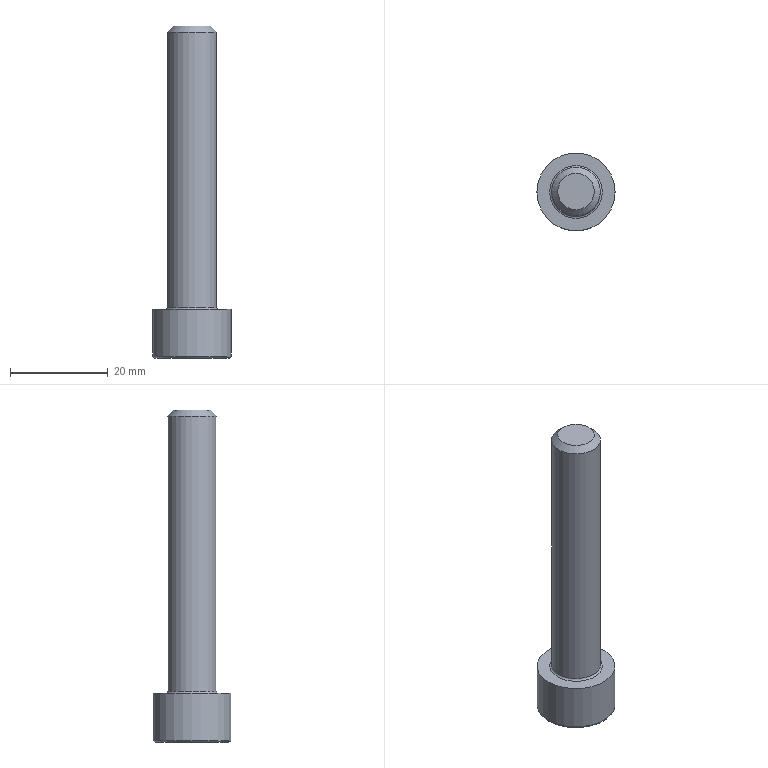Part | STEP file | solid 158 | 1 solid | 15 faces | box 16 x 16 x 68 mm | volume 6266 mm3 | plane 10 | cylinder 2 | torus 2 | cone 1 | commonest cylinder face diameters 10 x1 16 x1